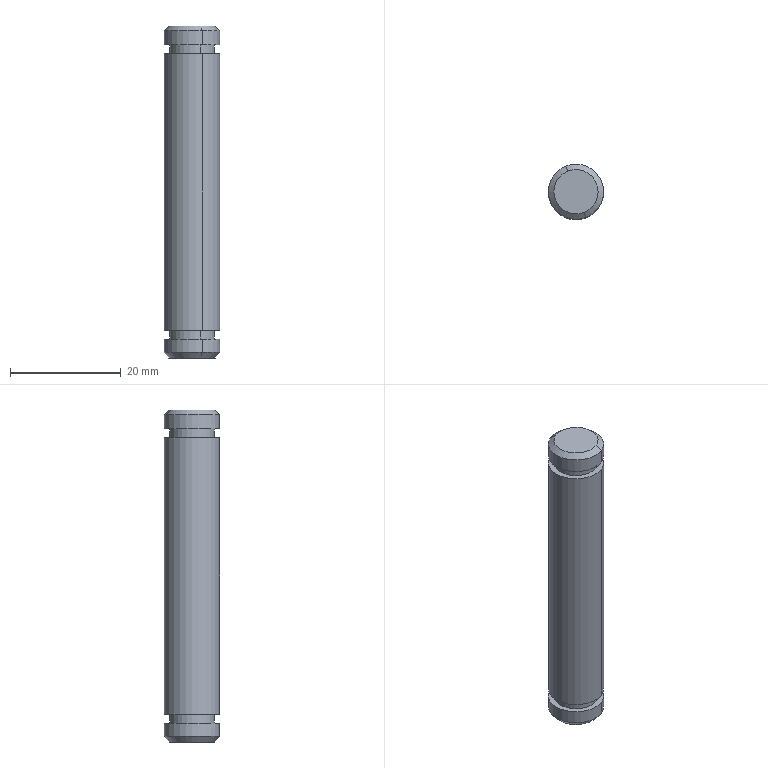Part | NX | features BREP 1 | 1 solid | 20 faces | box 10 x 10 x 60 mm | volume 4597 mm3 | cylinder 10 | plane 6 | cone 4 | commonest cylinder face diameters 10 x6 8 x4
STEP:
#1=CARTESIAN_POINT('',(-125.477,254.226,30.));
#2=VERTEX_POINT('',#1);
#3=CARTESIAN_POINT('',(-122.523,246.791,30.));
#4=VERTEX_POINT('',#3);
#5=CARTESIAN_POINT('',(-124.,250.509,30.));
#6=DIRECTION('',(0.,0.,1.));
#7=DIRECTION('',(-0.3692,0.9294,0.));
#8=AXIS2_PLACEMENT_3D('',#5,#6,#7);
#9=CIRCLE('',#8,4.);
#10=EDGE_CURVE('',#2,#4,#9,.T.);
#11=ORIENTED_EDGE('',*,*,#10,.F.);
#12=CARTESIAN_POINT('',(-125.846,255.155,29.161));
#13=VERTEX_POINT('',#12);
#14=CARTESIAN_POINT('',(-125.846,255.155,29.161));
#15=DIRECTION('',(0.2828,-0.7119,0.6428));
#16=VECTOR('',#15,1000.);
#17=LINE('',#14,#16);
#18=EDGE_CURVE('',#13,#2,#17,.T.);
#19=ORIENTED_EDGE('',*,*,#18,.F.);
#20=CARTESIAN_POINT('',(-122.154,245.862,29.161));
#21=VERTEX_POINT('',#20);
#22=CARTESIAN_POINT('',(-124.,250.509,29.161));
#23=DIRECTION('',(0.,0.,-1.));
#24=DIRECTION('',(-0.3692,0.9294,0.));
#25=AXIS2_PLACEMENT_3D('',#22,#23,#24);
#26=CIRCLE('',#25,5.);
#27=EDGE_CURVE('',#21,#13,#26,.T.);
#28=ORIENTED_EDGE('',*,*,#27,.F.);
#29=CARTESIAN_POINT('',(-122.154,245.862,29.161));
#30=DIRECTION('',(0.2828,-0.7119,-0.6428));
#31=VECTOR('',#30,1000.);
#32=LINE('',#29,#31);
#33=EDGE_CURVE('',#4,#21,#32,.T.);
#34=ORIENTED_EDGE('',*,*,#33,.F.);
#35=EDGE_LOOP('',(#11,#19,#28,#34));
#36=FACE_BOUND('',#35,.T.);
#37=CARTESIAN_POINT('',(-124.,250.509,29.161));
#38=DIRECTION('',(0.,0.,-1.));
#39=DIRECTION('',(-0.3692,0.9294,0.));
#40=AXIS2_PLACEMENT_3D('',#37,#38,#39);
#41=CONICAL_SURFACE('',#40,5.,0.8727);
#42=ADVANCED_FACE('',(#36),#41,.T.);
#43=CARTESIAN_POINT('',(-122.464,246.642,-30.));
#44=VERTEX_POINT('',#43);
#45=CARTESIAN_POINT('',(-125.536,254.376,-30.));
#46=VERTEX_POINT('',#45);
#47=CARTESIAN_POINT('',(-124.,250.509,-30.));
#48=DIRECTION('',(0.,0.,-1.));
#49=DIRECTION('',(0.3692,-0.9294,0.));
#50=AXIS2_PLACEMENT_3D('',#47,#48,#49);
#51=CIRCLE('',#50,4.161);
#52=EDGE_CURVE('',#44,#46,#51,.T.);
#53=ORIENTED_EDGE('',*,*,#52,.F.);
#54=CARTESIAN_POINT('',(-122.154,245.862,-29.));
#55=VERTEX_POINT('',#54);
#56=CARTESIAN_POINT('',(-122.464,246.642,-30.));
#57=DIRECTION('',(0.2373,-0.5974,0.766));
#58=VECTOR('',#57,1000.);
#59=LINE('',#56,#58);
#60=EDGE_CURVE('',#44,#55,#59,.T.);
#61=ORIENTED_EDGE('',*,*,#60,.T.);
#62=CARTESIAN_POINT('',(-125.846,255.155,-29.));
#63=VERTEX_POINT('',#62);
#64=CARTESIAN_POINT('',(-124.,250.509,-29.));
#65=DIRECTION('',(0.,0.,1.));
#66=DIRECTION('',(0.3692,-0.9294,0.));
#67=AXIS2_PLACEMENT_3D('',#64,#65,#66);
#68=CIRCLE('',#67,5.);
#69=EDGE_CURVE('',#63,#55,#68,.T.);
#70=ORIENTED_EDGE('',*,*,#69,.F.);
#71=CARTESIAN_POINT('',(-125.536,254.376,-30.));
#72=DIRECTION('',(0.2373,-0.5974,-0.766));
#73=VECTOR('',#72,1000.);
#74=LINE('',#71,#73);
#75=EDGE_CURVE('',#63,#46,#74,.T.);
#76=ORIENTED_EDGE('',*,*,#75,.T.);
#77=EDGE_LOOP('',(#53,#61,#70,#76));
#78=FACE_BOUND('',#77,.T.);
#79=CARTESIAN_POINT('',(-124.,250.509,-30.));
#80=DIRECTION('',(0.,0.,1.));
#81=DIRECTION('',(0.3692,-0.9294,0.));
#82=AXIS2_PLACEMENT_3D('',#79,#80,#81);
#83=CONICAL_SURFACE('',#82,4.161,0.6981);
#84=ADVANCED_FACE('',(#78),#83,.T.);
#85=CARTESIAN_POINT('',(-125.846,255.155,26.6));
#86=VERTEX_POINT('',#85);
#87=CARTESIAN_POINT('',(-122.154,245.862,26.6));
#88=VERTEX_POINT('',#87);
#89=CARTESIAN_POINT('',(-124.,250.509,26.6));
#90=DIRECTION('',(0.,0.,1.));
#91=DIRECTION('',(-0.3692,0.9294,0.));
#92=AXIS2_PLACEMENT_3D('',#89,#90,#91);
#93=CIRCLE('',#92,5.);
#94=EDGE_CURVE('',#86,#88,#93,.T.);
#95=ORIENTED_EDGE('',*,*,#94,.T.);
#96=CARTESIAN_POINT('',(-122.154,245.862,-30.));
#97=DIRECTION('',(0.,0.,-1.));
#98=VECTOR('',#97,1000.);
#99=LINE('',#96,#98);
#100=EDGE_CURVE('',#21,#88,#99,.T.);
#101=ORIENTED_EDGE('',*,*,#100,.F.);
#102=ORIENTED_EDGE('',*,*,#27,.T.);
#103=CARTESIAN_POINT('',(-125.846,255.155,-30.));
#104=DIRECTION('',(0.,0.,1.));
#105=VECTOR('',#104,1000.);
#106=LINE('',#103,#105);
#107=EDGE_CURVE('',#86,#13,#106,.T.);
#108=ORIENTED_EDGE('',*,*,#107,.F.);
#109=EDGE_LOOP('',(#95,#101,#102,#108));
#110=FACE_BOUND('',#109,.T.);
#111=CARTESIAN_POINT('',(-124.,250.509,-30.));
#112=DIRECTION('',(0.,0.,1.));
#113=DIRECTION('',(0.3692,-0.9294,0.));
#114=AXIS2_PLACEMENT_3D('',#111,#112,#113);
#115=CYLINDRICAL_SURFACE('',#114,5.);
#116=ADVANCED_FACE('',(#110),#115,.T.);
#117=CARTESIAN_POINT('',(-125.477,254.226,26.6));
#118=VERTEX_POINT('',#117);
#119=CARTESIAN_POINT('',(-122.523,246.791,26.6));
#120=VERTEX_POINT('',#119);
#121=CARTESIAN_POINT('',(-124.,250.509,26.6));
#122=DIRECTION('',(0.,0.,1.));
#123=DIRECTION('',(-0.3692,0.9294,0.));
#124=AXIS2_PLACEMENT_3D('',#121,#122,#123);
#125=CIRCLE('',#124,4.);
#126=EDGE_CURVE('',#118,#120,#125,.T.);
#127=ORIENTED_EDGE('',*,*,#126,.F.);
#128=CARTESIAN_POINT('',(-125.477,254.226,25.));
#129=VERTEX_POINT('',#128);
#130=CARTESIAN_POINT('',(-125.477,254.226,26.6));
#131=DIRECTION('',(0.,0.,-1.));
#132=VECTOR('',#131,1000.);
#133=LINE('',#130,#132);
#134=EDGE_CURVE('',#118,#129,#133,.T.);
#135=ORIENTED_EDGE('',*,*,#134,.T.);
#136=CARTESIAN_POINT('',(-122.523,246.791,25.));
#137=VERTEX_POINT('',#136);
#138=CARTESIAN_POINT('',(-124.,250.509,25.));
#139=DIRECTION('',(0.,0.,1.));
#140=DIRECTION('',(-0.3692,0.9294,0.));
#141=AXIS2_PLACEMENT_3D('',#138,#139,#140);
#142=CIRCLE('',#141,4.);
#143=EDGE_CURVE('',#129,#137,#142,.T.);
#144=ORIENTED_EDGE('',*,*,#143,.T.);
#145=CARTESIAN_POINT('',(-122.523,246.791,26.6));
#146=DIRECTION('',(0.,0.,1.));
#147=VECTOR('',#146,1000.);
#148=LINE('',#145,#147);
#149=EDGE_CURVE('',#137,#120,#148,.T.);
#150=ORIENTED_EDGE('',*,*,#149,.T.);
#151=EDGE_LOOP('',(#127,#135,#144,#150));
#152=FACE_BOUND('',#151,.T.);
#153=CARTESIAN_POINT('',(-124.,250.509,26.6));
#154=DIRECTION('',(0.,0.,-1.));
#155=DIRECTION('',(-0.3692,0.9294,0.));
#156=AXIS2_PLACEMENT_3D('',#153,#154,#155);
#157=CYLINDRICAL_SURFACE('',#156,4.);
#158=ADVANCED_FACE('',(#152),#157,.T.);
#159=CARTESIAN_POINT('',(-125.846,255.155,-25.));
#160=VERTEX_POINT('',#159);
#161=CARTESIAN_POINT('',(-122.154,245.862,-25.));
#162=VERTEX_POINT('',#161);
#163=CARTESIAN_POINT('',(-124.,250.509,-25.));
#164=DIRECTION('',(0.,0.,1.));
#165=DIRECTION('',(-0.3692,0.9294,0.));
#166=AXIS2_PLACEMENT_3D('',#163,#164,#165);
#167=CIRCLE('',#166,5.);
#168=EDGE_CURVE('',#160,#162,#167,.T.);
#169=ORIENTED_EDGE('',*,*,#168,.T.);
#170=CARTESIAN_POINT('',(-122.154,245.862,25.));
#171=VERTEX_POINT('',#170);
#172=CARTESIAN_POINT('',(-122.154,245.862,-30.));
#173=DIRECTION('',(0.,0.,1.));
#174=VECTOR('',#173,1000.);
#175=LINE('',#172,#174);
#176=EDGE_CURVE('',#162,#171,#175,.T.);
#177=ORIENTED_EDGE('',*,*,#176,.T.);
#178=CARTESIAN_POINT('',(-125.846,255.155,25.));
#179=VERTEX_POINT('',#178);
#180=CARTESIAN_POINT('',(-124.,250.509,25.));
#181=DIRECTION('',(0.,0.,1.));
#182=DIRECTION('',(-0.3692,0.9294,0.));
#183=AXIS2_PLACEMENT_3D('',#180,#181,#182);
#184=CIRCLE('',#183,5.);
#185=EDGE_CURVE('',#179,#171,#184,.T.);
#186=ORIENTED_EDGE('',*,*,#185,.F.);
#187=CARTESIAN_POINT('',(-125.846,255.155,-30.));
#188=DIRECTION('',(0.,0.,-1.));
#189=VECTOR('',#188,1000.);
#190=LINE('',#187,#189);
#191=EDGE_CURVE('',#179,#160,#190,.T.);
#192=ORIENTED_EDGE('',*,*,#191,.T.);
#193=EDGE_LOOP('',(#169,#177,#186,#192));
#194=FACE_BOUND('',#193,.T.);
#195=CARTESIAN_POINT('',(-124.,250.509,-30.));
#196=DIRECTION('',(0.,0.,1.));
#197=DIRECTION('',(0.3692,-0.9294,0.));
#198=AXIS2_PLACEMENT_3D('',#195,#196,#197);
#199=CYLINDRICAL_SURFACE('',#198,5.);
#200=ADVANCED_FACE('',(#194),#199,.T.);
#201=CARTESIAN_POINT('',(-125.477,254.226,-26.6));
#202=VERTEX_POINT('',#201);
#203=CARTESIAN_POINT('',(-122.523,246.791,-26.6));
#204=VERTEX_POINT('',#203);
#205=CARTESIAN_POINT('',(-124.,250.509,-26.6));
#206=DIRECTION('',(0.,0.,1.));
#207=DIRECTION('',(-0.3692,0.9294,0.));
#208=AXIS2_PLACEMENT_3D('',#205,#206,#207);
#209=CIRCLE('',#208,4.);
#210=EDGE_CURVE('',#202,#204,#209,.T.);
#211=ORIENTED_EDGE('',*,*,#210,.T.);
#212=CARTESIAN_POINT('',(-122.523,246.791,-25.));
#213=VERTEX_POINT('',#212);
#214=CARTESIAN_POINT('',(-122.523,246.791,-26.6));
#215=DIRECTION('',(0.,0.,1.));
#216=VECTOR('',#215,1000.);
#217=LINE('',#214,#216);
#218=EDGE_CURVE('',#204,#213,#217,.T.);
#219=ORIENTED_EDGE('',*,*,#218,.T.);
#220=CARTESIAN_POINT('',(-125.477,254.226,-25.));
#221=VERTEX_POINT('',#220);
#222=CARTESIAN_POINT('',(-124.,250.509,-25.));
#223=DIRECTION('',(0.,0.,1.));
#224=DIRECTION('',(-0.3692,0.9294,0.));
#225=AXIS2_PLACEMENT_3D('',#222,#223,#224);
#226=CIRCLE('',#225,4.);
#227=EDGE_CURVE('',#221,#213,#226,.T.);
#228=ORIENTED_EDGE('',*,*,#227,.F.);
#229=CARTESIAN_POINT('',(-125.477,254.226,-26.6));
#230=DIRECTION('',(0.,0.,-1.));
#231=VECTOR('',#230,1000.);
#232=LINE('',#229,#231);
#233=EDGE_CURVE('',#221,#202,#232,.T.);
#234=ORIENTED_EDGE('',*,*,#233,.T.);
#235=EDGE_LOOP('',(#211,#219,#228,#234));
#236=FACE_BOUND('',#235,.T.);
#237=CARTESIAN_POINT('',(-124.,250.509,-26.6));
#238=DIRECTION('',(0.,0.,1.));
#239=DIRECTION('',(0.3692,-0.9294,0.));
#240=AXIS2_PLACEMENT_3D('',#237,#238,#239);
#241=CYLINDRICAL_SURFACE('',#240,4.);
#242=ADVANCED_FACE('',(#236),#241,.T.);
#243=ORIENTED_EDGE('',*,*,#69,.T.);
#244=CARTESIAN_POINT('',(-122.154,245.862,-26.6));
#245=VERTEX_POINT('',#244);
#246=CARTESIAN_POINT('',(-122.154,245.862,-30.));
#247=DIRECTION('',(0.,0.,-1.));
#248=VECTOR('',#247,1000.);
#249=LINE('',#246,#248);
#250=EDGE_CURVE('',#245,#55,#249,.T.);
#251=ORIENTED_EDGE('',*,*,#250,.F.);
#252=CARTESIAN_POINT('',(-125.846,255.155,-26.6));
#253=VERTEX_POINT('',#252);
#254=CARTESIAN_POINT('',(-124.,250.509,-26.6));
#255=DIRECTION('',(0.,0.,1.));
#256=DIRECTION('',(-0.3692,0.9294,0.));
#257=AXIS2_PLACEMENT_3D('',#254,#255,#256);
#258=CIRCLE('',#257,5.);
#259=EDGE_CURVE('',#253,#245,#258,.T.);
#260=ORIENTED_EDGE('',*,*,#259,.F.);
#261=CARTESIAN_POINT('',(-125.846,255.155,-30.));
#262=DIRECTION('',(0.,0.,1.));
#263=VECTOR('',#262,1000.);
#264=LINE('',#261,#263);
#265=EDGE_CURVE('',#63,#253,#264,.T.);
#266=ORIENTED_EDGE('',*,*,#265,.F.);
#267=EDGE_LOOP('',(#243,#251,#260,#266));
#268=FACE_BOUND('',#267,.T.);
#269=CARTESIAN_POINT('',(-124.,250.509,-30.));
#270=DIRECTION('',(0.,0.,1.));
#271=DIRECTION('',(0.3692,-0.9294,0.));
#272=AXIS2_PLACEMENT_3D('',#269,#270,#271);
#273=CYLINDRICAL_SURFACE('',#272,5.);
#274=ADVANCED_FACE('',(#268),#273,.T.);
#275=ORIENTED_EDGE('',*,*,#250,.T.);
#276=CARTESIAN_POINT('',(-124.,250.509,-29.));
#277=DIRECTION('',(0.,0.,1.));
#278=DIRECTION('',(0.3692,-0.9294,0.));
#279=AXIS2_PLACEMENT_3D('',#276,#277,#278);
#280=CIRCLE('',#279,5.);
#281=EDGE_CURVE('',#55,#63,#280,.T.);
#282=ORIENTED_EDGE('',*,*,#281,.T.);
#283=ORIENTED_EDGE('',*,*,#265,.T.);
#284=CARTESIAN_POINT('',(-124.,250.509,-26.6));
#285=DIRECTION('',(0.,0.,1.));
#286=DIRECTION('',(-0.3692,0.9294,0.));
#287=AXIS2_PLACEMENT_3D('',#284,#285,#286);
#288=CIRCLE('',#287,5.);
#289=EDGE_CURVE('',#245,#253,#288,.T.);
#290=ORIENTED_EDGE('',*,*,#289,.F.);
#291=EDGE_LOOP('',(#275,#282,#283,#290));
#292=FACE_BOUND('',#291,.T.);
#293=CARTESIAN_POINT('',(-124.,250.509,-30.));
#294=DIRECTION('',(0.,0.,1.));
#295=DIRECTION('',(0.3692,-0.9294,0.));
#296=AXIS2_PLACEMENT_3D('',#293,#294,#295);
#297=CYLINDRICAL_SURFACE('',#296,5.);
#298=ADVANCED_FACE('',(#292),#297,.T.);
#299=CARTESIAN_POINT('',(-124.,250.509,-30.));
#300=DIRECTION('',(0.,0.,-1.));
#301=DIRECTION('',(0.3692,-0.9294,0.));
#302=AXIS2_PLACEMENT_3D('',#299,#300,#301);
#303=CIRCLE('',#302,4.161);
#304=EDGE_CURVE('',#46,#44,#303,.T.);
#305=ORIENTED_EDGE('',*,*,#304,.T.);
#306=ORIENTED_EDGE('',*,*,#52,.T.);
#307=EDGE_LOOP('',(#305,#306));
#308=FACE_BOUND('',#307,.T.);
#309=CARTESIAN_POINT('',(-124.,250.509,-30.));
#310=DIRECTION('',(0.,0.,-1.));
#311=DIRECTION('',(-0.3692,0.9294,0.));
#312=AXIS2_PLACEMENT_3D('',#309,#310,#311);
#313=PLANE('',#312);
#314=ADVANCED_FACE('',(#308),#313,.T.);
#315=ORIENTED_EDGE('',*,*,#210,.F.);
#316=CARTESIAN_POINT('',(-124.,250.509,-26.6));
#317=DIRECTION('',(0.,0.,1.));
#318=DIRECTION('',(-0.3692,0.9294,0.));
#319=AXIS2_PLACEMENT_3D('',#316,#317,#318);
#320=CIRCLE('',#319,4.);
#321=EDGE_CURVE('',#204,#202,#320,.T.);
#322=ORIENTED_EDGE('',*,*,#321,.F.);
#323=EDGE_LOOP('',(#315,#322));
#324=FACE_BOUND('',#323,.T.);
#325=ORIENTED_EDGE('',*,*,#259,.T.);
#326=ORIENTED_EDGE('',*,*,#289,.T.);
#327=EDGE_LOOP('',(#325,#326));
#328=FACE_BOUND('',#327,.T.);
#329=CARTESIAN_POINT('',(-124.,250.509,-26.6));
#330=DIRECTION('',(0.,0.,1.));
#331=DIRECTION('',(0.3692,-0.9294,0.));
#332=AXIS2_PLACEMENT_3D('',#329,#330,#331);
#333=PLANE('',#332);
#334=ADVANCED_FACE('',(#324,#328),#333,.T.);
#335=ORIENTED_EDGE('',*,*,#227,.T.);
#336=CARTESIAN_POINT('',(-124.,250.509,-25.));
#337=DIRECTION('',(0.,0.,1.));
#338=DIRECTION('',(-0.3692,0.9294,0.));
#339=AXIS2_PLACEMENT_3D('',#336,#337,#338);
#340=CIRCLE('',#339,4.);
#341=EDGE_CURVE('',#213,#221,#340,.T.);
#342=ORIENTED_EDGE('',*,*,#341,.T.);
#343=EDGE_LOOP('',(#335,#342));
#344=FACE_BOUND('',#343,.T.);
#345=ORIENTED_EDGE('',*,*,#168,.F.);
#346=CARTESIAN_POINT('',(-124.,250.509,-25.));
#347=DIRECTION('',(0.,0.,1.));
#348=DIRECTION('',(-0.3692,0.9294,0.));
#349=AXIS2_PLACEMENT_3D('',#346,#347,#348);
#350=CIRCLE('',#349,5.);
#351=EDGE_CURVE('',#162,#160,#350,.T.);
#352=ORIENTED_EDGE('',*,*,#351,.F.);
#353=EDGE_LOOP('',(#345,#352));
#354=FACE_BOUND('',#353,.T.);
#355=CARTESIAN_POINT('',(-124.,250.509,-25.));
#356=DIRECTION('',(0.,0.,1.));
#357=DIRECTION('',(0.3692,-0.9294,0.));
#358=AXIS2_PLACEMENT_3D('',#355,#356,#357);
#359=PLANE('',#358);
#360=ADVANCED_FACE('',(#344,#354),#359,.F.);
#361=ORIENTED_EDGE('',*,*,#218,.F.);
#362=ORIENTED_EDGE('',*,*,#321,.T.);
#363=ORIENTED_EDGE('',*,*,#233,.F.);
#364=ORIENTED_EDGE('',*,*,#341,.F.);
#365=EDGE_LOOP('',(#361,#362,#363,#364));
#366=FACE_BOUND('',#365,.T.);
#367=CARTESIAN_POINT('',(-124.,250.509,-26.6));
#368=DIRECTION('',(0.,0.,1.));
#369=DIRECTION('',(0.3692,-0.9294,0.));
#370=AXIS2_PLACEMENT_3D('',#367,#368,#369);
#371=CYLINDRICAL_SURFACE('',#370,4.);
#372=ADVANCED_FACE('',(#366),#371,.T.);
#373=ORIENTED_EDGE('',*,*,#176,.F.);
#374=ORIENTED_EDGE('',*,*,#351,.T.);
#375=ORIENTED_EDGE('',*,*,#191,.F.);
#376=CARTESIAN_POINT('',(-124.,250.509,25.));
#377=DIRECTION('',(0.,0.,1.));
#378=DIRECTION('',(-0.3692,0.9294,0.));
#379=AXIS2_PLACEMENT_3D('',#376,#377,#378);
#380=CIRCLE('',#379,5.);
#381=EDGE_CURVE('',#171,#179,#380,.T.);
#382=ORIENTED_EDGE('',*,*,#381,.F.);
#383=EDGE_LOOP('',(#373,#374,#375,#382));
#384=FACE_BOUND('',#383,.T.);
#385=CARTESIAN_POINT('',(-124.,250.509,-30.));
#386=DIRECTION('',(0.,0.,1.));
#387=DIRECTION('',(0.3692,-0.9294,0.));
#388=AXIS2_PLACEMENT_3D('',#385,#386,#387);
#389=CYLINDRICAL_SURFACE('',#388,5.);
#390=ADVANCED_FACE('',(#384),#389,.T.);
#391=ORIENTED_EDGE('',*,*,#94,.F.);
#392=CARTESIAN_POINT('',(-124.,250.509,26.6));
#393=DIRECTION('',(0.,0.,1.));
#394=DIRECTION('',(-0.3692,0.9294,0.));
#395=AXIS2_PLACEMENT_3D('',#392,#393,#394);
#396=CIRCLE('',#395,5.);
#397=EDGE_CURVE('',#88,#86,#396,.T.);
#398=ORIENTED_EDGE('',*,*,#397,.F.);
#399=EDGE_LOOP('',(#391,#398));
#400=FACE_BOUND('',#399,.T.);
#401=CARTESIAN_POINT('',(-124.,250.509,26.6));
#402=DIRECTION('',(0.,0.,1.));
#403=DIRECTION('',(-0.3692,0.9294,0.));
#404=AXIS2_PLACEMENT_3D('',#401,#402,#403);
#405=CIRCLE('',#404,4.);
#406=EDGE_CURVE('',#120,#118,#405,.T.);
#407=ORIENTED_EDGE('',*,*,#406,.T.);
#408=ORIENTED_EDGE('',*,*,#126,.T.);
#409=EDGE_LOOP('',(#407,#408));
#410=FACE_BOUND('',#409,.T.);
#411=CARTESIAN_POINT('',(-124.,250.509,26.6));
#412=DIRECTION('',(0.,0.,-1.));
#413=DIRECTION('',(0.3692,-0.9294,0.));
#414=AXIS2_PLACEMENT_3D('',#411,#412,#413);
#415=PLANE('',#414);
#416=ADVANCED_FACE('',(#400,#410),#415,.T.);
#417=ORIENTED_EDGE('',*,*,#185,.T.);
#418=ORIENTED_EDGE('',*,*,#381,.T.);
#419=EDGE_LOOP('',(#417,#418));
#420=FACE_BOUND('',#419,.T.);
#421=CARTESIAN_POINT('',(-124.,250.509,25.));
#422=DIRECTION('',(0.,0.,1.));
#423=DIRECTION('',(-0.3692,0.9294,0.));
#424=AXIS2_PLACEMENT_3D('',#421,#422,#423);
#425=CIRCLE('',#424,4.);
#426=EDGE_CURVE('',#137,#129,#425,.T.);
#427=ORIENTED_EDGE('',*,*,#426,.F.);
#428=ORIENTED_EDGE('',*,*,#143,.F.);
#429=EDGE_LOOP('',(#427,#428));
#430=FACE_BOUND('',#429,.T.);
#431=CARTESIAN_POINT('',(-124.,250.509,25.));
#432=DIRECTION('',(0.,0.,-1.));
#433=DIRECTION('',(0.3692,-0.9294,0.));
#434=AXIS2_PLACEMENT_3D('',#431,#432,#433);
#435=PLANE('',#434);
#436=ADVANCED_FACE('',(#420,#430),#435,.F.);
#437=ORIENTED_EDGE('',*,*,#134,.F.);
#438=ORIENTED_EDGE('',*,*,#406,.F.);
#439=ORIENTED_EDGE('',*,*,#149,.F.);
#440=ORIENTED_EDGE('',*,*,#426,.T.);
#441=EDGE_LOOP('',(#437,#438,#439,#440));
#442=FACE_BOUND('',#441,.T.);
#443=CARTESIAN_POINT('',(-124.,250.509,26.6));
#444=DIRECTION('',(0.,0.,-1.));
#445=DIRECTION('',(-0.3692,0.9294,0.));
#446=AXIS2_PLACEMENT_3D('',#443,#444,#445);
#447=CYLINDRICAL_SURFACE('',#446,4.);
#448=ADVANCED_FACE('',(#442),#447,.T.);
#449=CARTESIAN_POINT('',(-124.,250.509,30.));
#450=DIRECTION('',(0.,0.,1.));
#451=DIRECTION('',(-0.3692,0.9294,0.));
#452=AXIS2_PLACEMENT_3D('',#449,#450,#451);
#453=CIRCLE('',#452,4.);
#454=EDGE_CURVE('',#4,#2,#453,.T.);
#455=ORIENTED_EDGE('',*,*,#454,.T.);
#456=ORIENTED_EDGE('',*,*,#10,.T.);
#457=EDGE_LOOP('',(#455,#456));
#458=FACE_BOUND('',#457,.T.);
#459=CARTESIAN_POINT('',(-124.,250.509,30.));
#460=DIRECTION('',(0.,0.,1.));
#461=DIRECTION('',(-0.3692,0.9294,0.));
#462=AXIS2_PLACEMENT_3D('',#459,#460,#461);
#463=PLANE('',#462);
#464=ADVANCED_FACE('',(#458),#463,.T.);
#465=ORIENTED_EDGE('',*,*,#100,.T.);
#466=ORIENTED_EDGE('',*,*,#397,.T.);
#467=ORIENTED_EDGE('',*,*,#107,.T.);
#468=CARTESIAN_POINT('',(-124.,250.509,29.161));
#469=DIRECTION('',(0.,0.,-1.));
#470=DIRECTION('',(-0.3692,0.9294,0.));
#471=AXIS2_PLACEMENT_3D('',#468,#469,#470);
#472=CIRCLE('',#471,5.);
#473=EDGE_CURVE('',#13,#21,#472,.T.);
#474=ORIENTED_EDGE('',*,*,#473,.T.);
#475=EDGE_LOOP('',(#465,#466,#467,#474));
#476=FACE_BOUND('',#475,.T.);
#477=CARTESIAN_POINT('',(-124.,250.509,-30.));
#478=DIRECTION('',(0.,0.,1.));
#479=DIRECTION('',(0.3692,-0.9294,0.));
#480=AXIS2_PLACEMENT_3D('',#477,#478,#479);
#481=CYLINDRICAL_SURFACE('',#480,5.);
#482=ADVANCED_FACE('',(#476),#481,.T.);
#483=ORIENTED_EDGE('',*,*,#60,.F.);
#484=ORIENTED_EDGE('',*,*,#304,.F.);
#485=ORIENTED_EDGE('',*,*,#75,.F.);
#486=ORIENTED_EDGE('',*,*,#281,.F.);
#487=EDGE_LOOP('',(#483,#484,#485,#486));
#488=FACE_BOUND('',#487,.T.);
#489=CARTESIAN_POINT('',(-124.,250.509,-30.));
#490=DIRECTION('',(0.,0.,1.));
#491=DIRECTION('',(0.3692,-0.9294,0.));
#492=AXIS2_PLACEMENT_3D('',#489,#490,#491);
#493=CONICAL_SURFACE('',#492,4.161,0.6981);
#494=ADVANCED_FACE('',(#488),#493,.T.);
#495=ORIENTED_EDGE('',*,*,#18,.T.);
#496=ORIENTED_EDGE('',*,*,#454,.F.);
#497=ORIENTED_EDGE('',*,*,#33,.T.);
#498=ORIENTED_EDGE('',*,*,#473,.F.);
#499=EDGE_LOOP('',(#495,#496,#497,#498));
#500=FACE_BOUND('',#499,.T.);
#501=CARTESIAN_POINT('',(-124.,250.509,29.161));
#502=DIRECTION('',(0.,0.,-1.));
#503=DIRECTION('',(-0.3692,0.9294,0.));
#504=AXIS2_PLACEMENT_3D('',#501,#502,#503);
#505=CONICAL_SURFACE('',#504,5.,0.8727);
#506=ADVANCED_FACE('',(#500),#505,.T.);
#507=CLOSED_SHELL('',(#42,#84,#116,#158,#200,#242,#274,#298,#314,#334,#360,#372,#390,#416,#436,#448,#464,#482,#494,#506));
#508=MANIFOLD_SOLID_BREP('',#507);
#509=(LENGTH_UNIT()NAMED_UNIT(*)SI_UNIT(.MILLI.,.METRE.));
#510=UNCERTAINTY_MEASURE_WITH_UNIT(LENGTH_MEASURE(0.00001),#509,'','');
#511=(NAMED_UNIT(*)PLANE_ANGLE_UNIT()SI_UNIT($,.RADIAN.));
#512=(NAMED_UNIT(*)SI_UNIT($,.STERADIAN.)SOLID_ANGLE_UNIT());
#513=(GEOMETRIC_REPRESENTATION_CONTEXT(3)GLOBAL_UNCERTAINTY_ASSIGNED_CONTEXT((#510))GLOBAL_UNIT_ASSIGNED_CONTEXT((#509,#511,#512))REPRESENTATION_CONTEXT('',''));
#514=ADVANCED_BREP_SHAPE_REPRESENTATION('',(#508),#513);